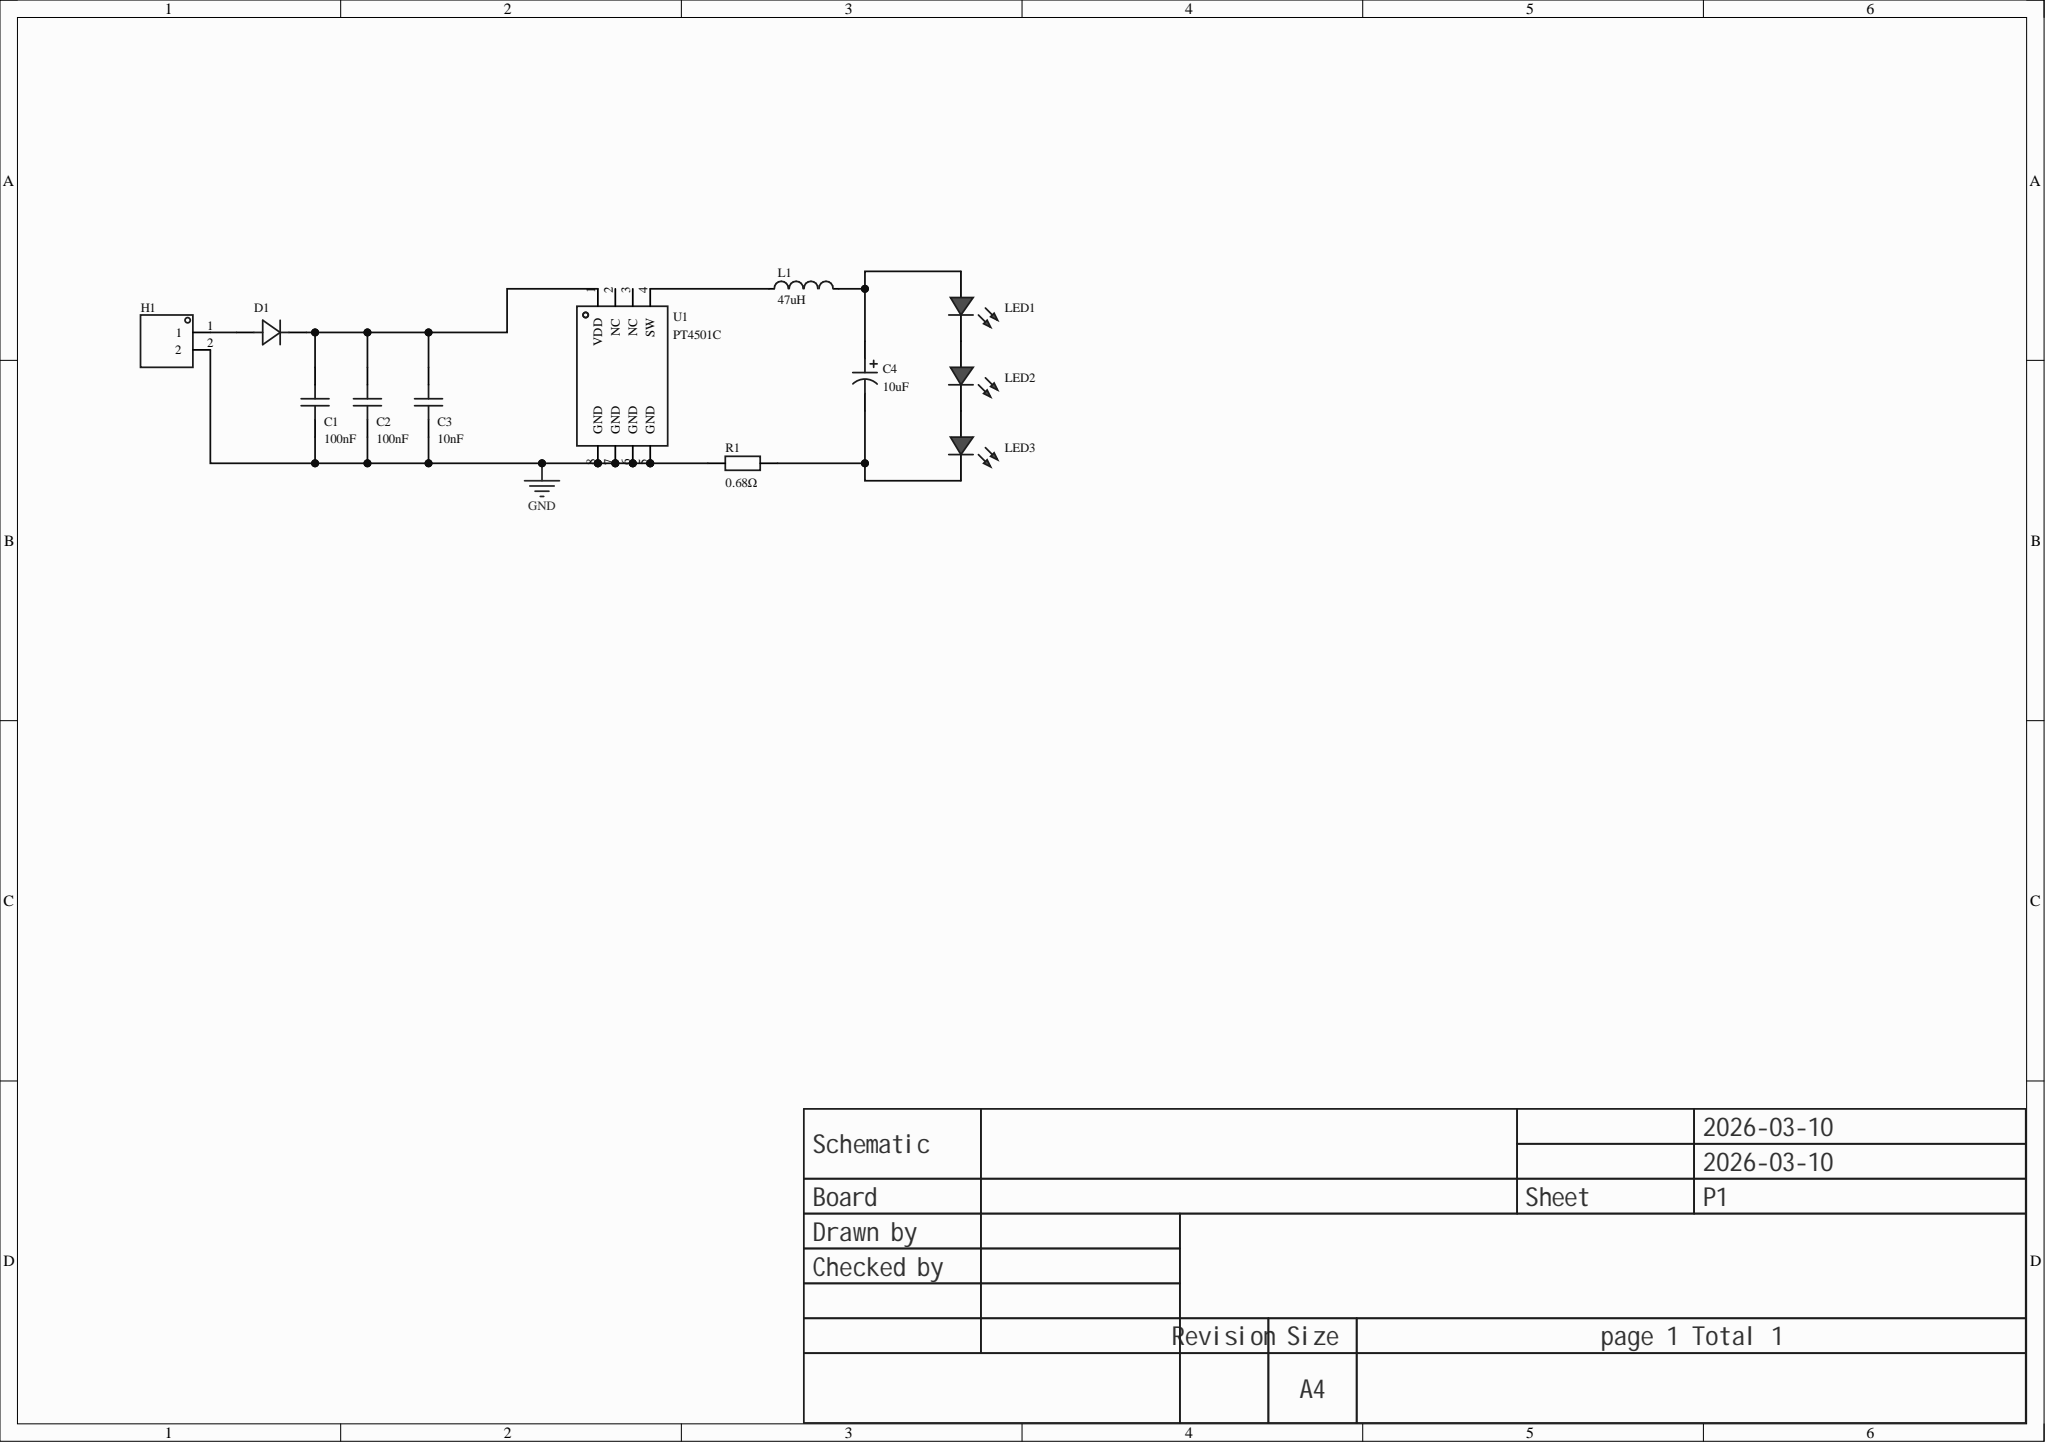Circuit board | Altium Designer | 12 parts | 8 nets
Bill of materials:
Comment,Description,Designator,Footprint,LibRef,Quantity
"100nF","","C1, C2","CAP-TH_L5.0-W2.5-P5.00-D1.0","100nF","2"
"10nF","","C3","CAP-TH_L5.0-W2.5-P5.00-D1.0","100nF","1"
"10uF","Capacitance: 10uF; Tolerance: ±20%; Rated voltage: 50V; Ripple current: 120mA@100KHz; Equivalent series resistance (ESR): 1.6Ω;","C4","CAP-TH_BD5.0-P2.00-D0.8-FD-10UF50VC110GL","10UF50VC110GL","1"
"","","D1","DO_1N4007","D_1N4007A","1"
"","","H1","HDR-TH_2P-P2.54-V-M-1","HDR-M_2.54_1x2P","1"
"47uH","Inductance: 47uH; Tolerance: ±15%; Rated current: 1.6A; Saturation current (Isat): -; Type: -; Quality factor: -;","L1","IND-TH_BD7.0-L17.8-P21.80-D0.8","IHD1RR470L","1"
"","","LED1, LED2, LED3","LED_TH-3mm","LED_TH-R_3mm","3"
"0.68Ω","","R1","Res_5W","Res_AXIAL-5W","1"
"PT4501C","Dual-channel single-stage linear LED driver IC","U1","SOP-8_L4.9-W3.9-P1.27-LS6.0-BL-EP","PT4516EESH","1"
Netlist (Protel format):
[
C1
CAP-TH_L5.0-W2.5-P5.00-D1.0
100nF



]
[
C2
CAP-TH_L5.0-W2.5-P5.00-D1.0
100nF



]
[
C3
CAP-TH_L5.0-W2.5-P5.00-D1.0
10nF



]
[
C4
CAP-TH_BD5.0-P2.00-D0.8-FD-10UF50VC110GL
10uF



]
[
D1
DO_1N4007




]
[
H1
HDR-TH_2P-P2.54-V-M-1




]
[
L1
IND-TH_BD7.0-L17.8-P21.80-D0.8
47uH



]
[
LED1
LED_TH-3mm




]
[
LED2
LED_TH-3mm




]
[
LED3
LED_TH-3mm




]
[
R1
Res_5W
0.68Ω



]
[
U1
SOP-8_L4.9-W3.9-P1.27-LS6.0-BL-EP
PT4501C



]
(
NetLED2_2
LED2-2
LED3-1
)
(
NetLED1_2
LED1-2
LED2-1
)
(
NetL1_1
L1-1
U1-4
)
(
NetD1_2
D1-2
H1-1
)
(
NetC4_2
C4-2
LED3-2
R1-2
)
(
NetC4_1
C4-1
L1-2
LED1-1
)
(
NetC1_1
C1-1
C2-1
C3-1
D1-1
U1-1
)
(
GND
C1-2
C2-2
C3-2
H1-2
R1-1
U1-5
U1-6
U1-7
U1-8
)